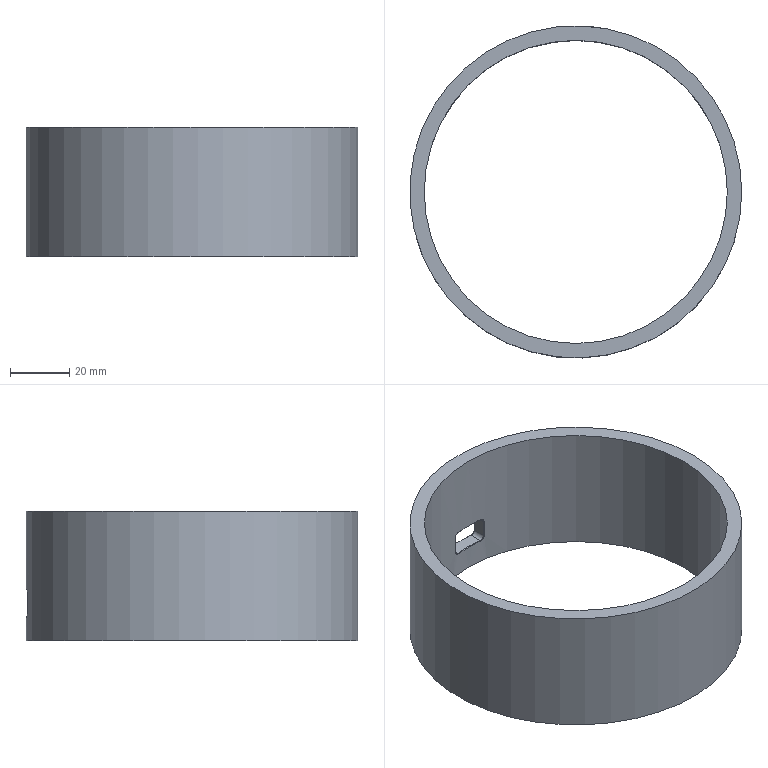NC program | NX | posted with a generic post | part box 112.5 x 112.5 x 44 mm
Whole program:
N10 G17 G21 G94 G90
(ZLEVEL_PROFILE_COPY , TOOL : D6)
N12 T04 M6
N14 G54
N16 G17 G0 G90 X1.72 Y10.5 B0. C0. S9500 M3
N18 G43 Z30. H4
N20 Z1.5
N22 G94 G1 X-3.75 Z1.213 F1500.
N24 Y8. Z1.082
N26 X3.75 Z0.689
N28 Y10.5 Z0.558
N30 X-3.75 Z0.165
N32 Y8. Z0.034
N34 X3.75 Z-0.359
N36 Y10.5 Z-0.49
N38 X-3.75
N40 Y8.
N42 X3.75
N44 Y10.5
N46 X-3.75 Z-0.735
N48 Y8. Z-0.817
N50 X1.25 Z-0.98
N52 X3.75
N54 Y10.5
N56 X-3.75 Z-1.225
N58 Y8. Z-1.306
N60 X1.25 Z-1.47
N62 X3.75
N64 Y10.5
N66 X-3.75 Z-1.715
N68 Y8. Z-1.796
N70 X1.25 Z-1.96
N72 X3.75
N74 Y10.5
N76 X-3.75 Z-2.205
N78 Y8. Z-2.286
N80 X1.25 Z-2.45
N82 X3.75
N84 Y10.5
N86 X-3.75 Z-2.695
N88 Y8. Z-2.776
N90 X1.25 Z-2.939
N92 X3.75
N94 Y10.5
N96 X-3.75 Z-3.184
N98 Y8. Z-3.266
N100 X1.25 Z-3.429
N102 X3.75
N104 Y10.5
N106 X-3.75 Z-3.674
N108 Y8. Z-3.756
N110 X1.25 Z-3.919
N112 X3.75
N114 Y10.5
N116 X-3.75 Z-4.164
N118 Y8. Z-4.246
N120 X1.25 Z-4.409
N122 X3.75
N124 Y10.5
N126 X-3.75 Z-4.654
N128 Y8. Z-4.736
N130 X1.25 Z-4.899
N132 X3.75
N134 Y10.5
N136 X-3.75 Z-5.144
N138 Y8. Z-5.226
N140 X1.25 Z-5.389
N142 X3.75
N144 Y10.5
N146 X-3.75 Z-5.634
N148 Y8. Z-5.716
N150 X1.25 Z-5.879
N152 X3.75
N154 Y10.5
N156 X-3.75 Z-6.124
N158 Y8. Z-6.206
N160 X1.25 Z-6.369
N162 X3.75
N164 Y10.5
N166 X-3.75
N168 Y8.
N170 X1.25
N172 Z-4.869
N174 G0 Z30.
N176 M5
(ADAPTIVE_MILLING , TOOL : D3)
N178 T05 M6
N180 G54
N182 G17 G0 G90 X3.003 Y7.25 B0. C0. S9500 M3
N184 G43 Z30. H5
N186 Z-3.
N188 G94 G1 Z-6. F1100.
N190 X3.197 Y6.702
N192 G3 X3.482 Y6.5 R0.305
N194 X4.28 Y6.992 R8.824
N196 X4.728 Y7.468 R2.682
N198 X5.201 Y8.025 R6.211
N200 X5.25 Y8.282 R0.441
N202 X4.998 Y8.603 R0.332
N204 X4.665 Y8.494 Z-5.939 R0.34
N206 G1 X4.503 Y8.33 Z-5.9
N208 X3.436 Y7.253
N210 X3.325 Y7.141 Z-5.926
N212 X3.217 Y7.026 Z-5.953
N214 G3 X3.161 Y6.756 Z-6. R0.335
N216 X3.482 Y6.5 R0.332
N218 X4.637 Y7.198 R2.342
N220 X5.198 Y7.85 R3.491
N222 G1 X5.238 Y7.919
N224 X5.25 Y7.998
N226 Y8.185
N228 G3 X4.694 Y8.426 R0.33
N230 G1 X3.256 Y7.07
N232 G3 X3.482 Y6.5 R0.33
N234 X4.253 Y6.758 R1.37
N236 X5.179 Y7.65 R3.378
N238 G1 X5.232 Y7.733
N240 X5.25 Y7.831
N242 Y8.
N244 G3 X4.705 Y8.25 R0.33
N246 G1 X3.342 Y7.08
N248 G3 X3.557 Y6.5 R0.33
N250 X4.37 Y6.739 R1.314
N252 X5.195 Y7.518 R2.602
N254 G1 X5.239 Y7.592
N256 X5.25 Y7.678
N258 Y7.847
N260 G3 X4.708 Y8.1 R0.33
N262 G1 X3.495 Y7.083
N264 G3 X3.707 Y6.5 R0.33
N266 X4.472 Y6.709 R1.272
N268 X5.216 Y7.408 R2.046
N270 X5.25 Y7.692 R0.614
N272 X4.71 Y7.946 R0.33
N274 G1 X3.666 Y7.085
N276 G3 X3.876 Y6.5 R0.33
N278 X4.654 Y6.73 R1.279
N280 X5.223 Y7.288 R1.579
N282 X5.25 Y7.536 R0.598
N284 X4.718 Y7.797 R0.33
N286 G1 X3.805 Y7.091
N288 G3 X4.007 Y6.5 R0.33
N290 X4.863 Y6.778 R1.276
N292 X5.234 Y7.191 R1.054
N294 X5.25 Y7.399 R0.714
N296 X4.723 Y7.664 R0.33
N298 G1 X3.96 Y7.094
N300 G3 X4.157 Y6.5 R0.33
N302 X5.086 Y6.871 R1.197
N304 X5.25 Y7.272 R0.457
N306 X4.727 Y7.54 R0.33
N308 G1 X4.114 Y7.098
N310 G3 X4.307 Y6.5 R0.33
N312 X5.22 Y6.95 R0.989
N314 X5.25 Y7.174 R0.509
N316 X4.723 Y7.439 R0.33
N318 G1 X4.26 Y7.095
N320 G3 X4.457 Y6.5 R0.33
N322 X5.216 Y6.859 R0.817
N324 X5.25 Y7.068 R0.434
N326 X4.728 Y7.336 R0.33
N328 G1 X4.396 Y7.098
N330 G3 X4.589 Y6.5 R0.33
N332 X5.218 Y6.794 R0.656
N334 G1 X5.248 Y6.852
N336 X5.259 Y6.917
N338 X5.25 Y6.982
N340 G3 X4.732 Y7.253 R0.33
N342 G1 X4.602 Y7.164
N344 X4.475 Y7.07
N346 G3 X4.701 Y6.5 R0.33
N348 X5.208 Y6.72 R0.54
N350 G1 X5.242 Y6.777
N352 X5.257 Y6.842
N354 X5.25 Y6.907
N356 G3 X4.747 Y7.188 R0.33
N358 G1 X4.663 Y7.137
N360 X4.581 Y7.081
N362 G3 X4.795 Y6.5 R0.33
N364 X5.205 Y6.673 R0.429
N366 G1 X5.239 Y6.727
N368 X5.255 Y6.789
N370 X5.25 Y6.853
N372 G3 X4.583 Y6.674 R-0.358
N374 X4.889 Y6.5 R0.359
N376 X5.25 Y6.828 R0.32
N378 X4.666 Y6.928 R0.301
N380 X5.009 Y6.508 R0.316
N382 G1 X5.027 Y6.514
N384 G3 X5.014 Y7.09 R0.303
N386 G1 X4.482 Y7.25
N388 Z-3.
N390 G0 Z30.
N392 X4.5 Y9.771
N394 Z-3.
N396 G1 Z-6.
N398 X5.04 Y9.944
N400 G3 X5.25 Y10.232 R0.305
N402 X4.758 Y11.03 R8.84
N404 X4.282 Y11.478 R2.677
N406 X3.725 Y11.951 R6.151
N408 X3.468 Y12. R0.441
N410 X3.147 Y11.748 R0.332
N412 X3.256 Y11.415 Z-5.939 R0.34
N414 G1 X3.42 Y11.253 Z-5.9
N416 X4.497 Y10.186
N418 X4.609 Y10.075 Z-5.926
N420 X4.724 Y9.967 Z-5.953
N422 G3 X4.994 Y9.911 Z-6. R0.335
N424 X5.25 Y10.232 R0.332
N426 X4.592 Y11.346 R2.271
N428 X3.916 Y11.938 R3.891
N430 G1 X3.84 Y11.986
N432 X3.752 Y12.
N434 X3.564
N436 G3 X3.324 Y11.444 R0.33
N438 G1 X4.68 Y10.006
N440 G3 X5.25 Y10.232 R0.33
N442 X5.002 Y10.987 R1.355
N444 X4.1 Y11.929 R3.388
N446 G1 X4.017 Y11.983
N448 X3.919 Y12.
N450 X3.75
N452 G3 X3.5 Y11.455 R0.33
N454 G1 X4.67 Y10.092
N456 G3 X5.25 Y10.307 R0.33
N458 X5.011 Y11.12 R1.315
N460 X4.232 Y11.945 R2.621
N462 G1 X4.158 Y11.989
N464 X4.072 Y12.
N466 X3.903
N468 G3 X3.65 Y11.458 R0.33
N470 G1 X4.667 Y10.245
N472 G3 X5.25 Y10.457 R0.33
N474 X5.04 Y11.222 R1.269
N476 X4.342 Y11.966 R2.047
N478 X4.058 Y12. R0.614
N480 X3.804 Y11.46 R0.33
N482 G1 X4.666 Y10.416
N484 G3 X5.25 Y10.626 R0.33
N486 X5.02 Y11.404 R1.279
N488 X4.462 Y11.973 R1.583
N490 X4.213 Y12. R0.597
N492 X3.954 Y11.465 R0.33
N494 G1 X4.661 Y10.572
N496 G3 X5.25 Y10.776 R0.33
N498 X4.983 Y11.597 R1.258
N500 X4.558 Y11.984 R1.07
N502 X4.351 Y12. R0.716
N504 X4.086 Y11.473 R0.33
N506 G1 X4.656 Y10.71
N508 G3 X5.25 Y10.907 R0.33
N510 X4.7 Y11.971 R1.184
N512 X4.477 Y12. R0.52
N514 X4.21 Y11.477 R0.33
N516 G1 X4.653 Y10.864
N518 G3 X5.25 Y11.057 R0.33
N520 X4.799 Y11.97 R0.99
N522 X4.576 Y12. R0.509
N524 X4.311 Y11.473 R0.33
N526 G1 X4.655 Y11.01
N528 G3 X5.25 Y11.207 R0.33
N530 X4.89 Y11.966 R0.82
N532 X4.682 Y12. R0.433
N534 X4.414 Y11.477 R0.33
N536 G1 X4.652 Y11.146
N538 G3 X5.25 Y11.339 R0.33
N540 X4.956 Y11.968 R0.657
N542 G1 X4.897 Y11.998
N544 X4.833 Y12.009
N546 X4.768 Y12.
N548 G3 X4.497 Y11.481 R0.33
N550 G1 X4.586 Y11.351
N552 X4.68 Y11.224
N554 G3 X5.25 Y11.451 R0.33
N556 X5.029 Y11.958 R0.541
N558 G1 X4.973 Y11.992
N560 X4.908 Y12.007
N562 X4.843 Y12.
N564 G3 X4.562 Y11.496 R0.33
N566 G1 X4.614 Y11.412
N568 X4.669 Y11.331
N570 G3 X5.25 Y11.545 R0.33
N572 X5.061 Y11.964 R0.421
N574 G1 X4.983 Y12.
N576 X4.897
N578 G3 X5.076 Y11.333 R-0.358
N580 X5.25 Y11.639 R0.359
N582 X4.922 Y12. R0.32
N584 X4.822 Y11.416 R0.301
N586 X5.242 Y11.759 R0.316
N588 G1 X5.236 Y11.777
N590 G3 X4.66 Y11.764 R0.303
N592 G1 X4.5 Y11.232
N594 Z-3.
N596 G0 Z30.
N598 X-3.003 Y11.25
N600 Z-3.
N602 G1 Z-6.
N604 X-3.197 Y11.798
N606 G3 X-3.482 Y12. R0.305
N608 X-4.28 Y11.508 R8.768
N610 X-4.728 Y11.031 R2.69
N612 X-5.201 Y10.475 R6.229
N614 X-5.25 Y10.218 R0.441
N616 X-4.998 Y9.897 R0.332
N618 X-4.665 Y10.006 Z-5.939 R0.34
N620 G1 X-4.503 Y10.17 Z-5.9
N622 X-3.436 Y11.247
N624 X-3.325 Y11.359 Z-5.926
N626 X-3.217 Y11.474 Z-5.953
N628 G3 X-3.161 Y11.744 Z-6. R0.335
N630 X-3.482 Y12. R0.332
N632 X-4.596 Y11.341 R2.266
N634 X-5.188 Y10.666 R3.896
N636 G1 X-5.236 Y10.59
N638 X-5.25 Y10.502
N640 Y10.314
N642 G3 X-4.694 Y10.074 R0.33
N644 G1 X-3.256 Y11.43
N646 G3 X-3.482 Y12. R0.33
N648 X-4.237 Y11.752 R1.354
N650 X-5.179 Y10.85 R3.409
N652 G1 X-5.233 Y10.767
N654 X-5.25 Y10.669
N656 Y10.5
N658 G3 X-4.705 Y10.25 R0.33
N660 G1 X-3.342 Y11.42
N662 G3 X-3.557 Y12. R0.33
N664 X-4.354 Y11.771 R1.297
N666 X-5.195 Y10.982 R2.635
N668 G1 X-5.239 Y10.908
N670 X-5.25 Y10.822
N672 Y10.653
N674 G3 X-4.708 Y10.4 R0.33
N676 G1 X-3.495 Y11.417
N678 G3 X-3.707 Y12. R0.33
N680 X-4.472 Y11.79 R1.271
N682 X-5.216 Y11.092 R2.049
N684 X-5.25 Y10.808 R0.614
N686 X-4.71 Y10.553 R0.33
N688 G1 X-3.666 Y11.416
N690 G3 X-3.876 Y12. R0.33
N692 X-4.654 Y11.77 R1.281
N694 X-5.223 Y11.212 R1.581
N696 X-5.25 Y10.963 R0.598
N698 X-4.718 Y10.702 R0.33
N700 G1 X-3.805 Y11.409
N702 G3 X-4.007 Y12. R0.33
N704 X-4.847 Y11.732 R1.266
N706 X-5.234 Y11.308 R1.07
N708 X-5.25 Y11.1 R0.715
N710 X-4.722 Y10.836 R0.33
N712 G1 X-3.96 Y11.406
N714 G3 X-4.157 Y12. R0.33
N716 X-5.221 Y11.45 R1.185
N718 X-5.25 Y11.227 R0.521
N720 X-4.727 Y10.96 R0.33
N722 G1 X-4.114 Y11.403
N724 G3 X-4.307 Y12. R0.33
N726 X-5.22 Y11.549 R0.99
N728 X-5.25 Y11.326 R0.509
N730 X-4.723 Y11.061 R0.33
N732 G1 X-4.26 Y11.405
N734 G3 X-4.457 Y12. R0.33
N736 X-5.216 Y11.641 R0.818
N738 X-5.25 Y11.432 R0.433
N740 X-4.727 Y11.164 R0.33
N742 G1 X-4.396 Y11.402
N744 G3 X-4.589 Y12. R0.33
N746 X-5.218 Y11.706 R0.657
N748 G1 X-5.248 Y11.648
N750 X-5.259 Y11.583
N752 X-5.25 Y11.518
N754 G3 X-4.732 Y11.247 R0.33
N756 G1 X-4.601 Y11.336
N758 X-4.475 Y11.43
N760 G3 X-4.701 Y12. R0.33
N762 X-5.208 Y11.78 R0.541
N764 X-5.25 Y11.574 R0.389
N766 X-4.699 Y11.329 R0.33
N768 G1 X-4.627 Y11.393
N770 X-4.558 Y11.461
N772 G3 X-4.814 Y12. R0.33
N774 X-5.241 Y11.741 R0.385
N776 G1 X-5.245 Y11.723
N778 X-5.248 Y11.704
N780 X-5.25 Y11.686
N782 Y11.648
N784 G3 X-4.56 Y11.779 R-0.358
N786 X-4.889 Y12. R0.357
N788 X-5.25 Y11.672 R0.32
N790 X-4.666 Y11.572 R0.301
N792 X-5.009 Y11.992 R0.316
N794 G1 X-5.027 Y11.986
N796 G3 X-5.014 Y11.41 R0.303
N798 G1 X-4.482 Y11.25
N800 Z-3.
N802 G0 Z30.
N804 X-4.5 Y8.729
N806 Z-3.
N808 G1 Z-6.
N810 X-5.04 Y8.556
N812 G3 X-5.25 Y8.268 R0.305
N814 X-4.747 Y7.455 R8.169
N816 X-4.31 Y7.046 R2.452
N818 X-3.741 Y6.559 R8.24
N820 X-3.468 Y6.5 R0.427
N822 X-3.147 Y6.752 R0.332
N824 X-3.256 Y7.085 Z-5.939 R0.34
N826 G1 X-3.42 Y7.247 Z-5.9
N828 X-4.497 Y8.314
N830 X-4.609 Y8.425 Z-5.926
N832 X-4.724 Y8.533 Z-5.953
N834 G3 X-4.994 Y8.589 Z-6. R0.335
N836 X-5.25 Y8.268 R0.332
N838 X-4.605 Y7.167 R2.24
N840 X-3.917 Y6.562 R3.951
N842 G1 X-3.84 Y6.514
N844 X-3.752 Y6.5
N846 X-3.564
N848 G3 X-3.324 Y7.056 R0.33
N850 G1 X-4.68 Y8.494
N852 G3 X-5.25 Y8.268 R0.33
N854 X-4.992 Y7.497 R1.367
N856 X-4.1 Y6.571 R3.398
N858 G1 X-4.017 Y6.517
N860 X-3.919 Y6.5
N862 X-3.751
N864 G3 X-3.5 Y7.045 R0.33
N866 G1 X-4.67 Y8.408
N868 G3 X-5.25 Y8.193 R0.33
N870 X-5.011 Y7.38 R1.312
N872 X-4.232 Y6.555 R2.621
N874 G1 X-4.158 Y6.511
N876 X-4.072 Y6.5
N878 X-3.903
N880 G3 X-3.65 Y7.042 R0.33
N882 G1 X-4.667 Y8.255
N884 G3 X-5.25 Y8.043 R0.33
N886 X-5.041 Y7.278 R1.274
N888 X-4.342 Y6.534 R2.051
N890 X-4.058 Y6.5 R0.615
N892 X-3.802 Y7.038 R0.33
N894 G1 X-4.664 Y8.1
N896 G3 X-5.25 Y7.893 R0.33
N898 X-5.02 Y7.096 R1.291
N900 X-4.462 Y6.527 R1.581
N902 X-4.213 Y6.5 R0.598
N904 X-3.952 Y7.032 R0.33
N906 G1 X-4.659 Y7.945
N908 G3 X-5.25 Y7.743 R0.33
N910 X-4.972 Y6.888 R1.278
N912 X-4.558 Y6.516 R1.059
N914 X-4.35 Y6.5 R0.713
N916 X-4.086 Y7.028 R0.33
N918 G1 X-4.656 Y7.79
N920 G3 X-5.25 Y7.593 R0.33
N922 X-4.905 Y6.691 R1.192
N924 X-4.59 Y6.5 R0.517
N926 G1 X-4.477
N928 G3 X-4.21 Y7.023 R0.33
N930 G1 X-4.653 Y7.636
N932 G3 X-5.25 Y7.443 R0.33
N934 X-4.799 Y6.53 R0.989
N936 X-4.576 Y6.5 R0.509
N938 X-4.311 Y7.027 R0.33
N940 G1 X-4.655 Y7.49
N942 G3 X-5.25 Y7.293 R0.33
N944 X-4.891 Y6.534 R0.818
N946 X-4.682 Y6.5 R0.433
N948 X-4.414 Y7.023 R0.33
N950 G1 X-4.652 Y7.354
N952 G3 X-5.25 Y7.161 R0.33
N954 X-4.956 Y6.532 R0.657
N956 G1 X-4.898 Y6.502
N958 X-4.833 Y6.491
N960 X-4.768 Y6.5
N962 G3 X-4.497 Y7.018 R0.33
N964 G1 X-4.586 Y7.149
N966 X-4.68 Y7.275
N968 G3 X-5.25 Y7.049 R0.33
N970 X-5.029 Y6.542 R0.54
N972 X-4.824 Y6.5 R0.39
N974 X-4.562 Y7.031 R0.33
N976 G1 X-4.625 Y7.114
N978 X-4.692 Y7.194
N980 G3 X-5.25 Y6.955 R0.33
N982 X-5.077 Y6.545 R0.429
N984 G1 X-5.024 Y6.511
N986 X-4.962 Y6.495
N988 X-4.898 Y6.5
N990 G3 X-5.029 Y7.19 R-0.358
N992 X-5.25 Y6.861 R0.357
N994 X-4.922 Y6.5 R0.32
N996 X-4.822 Y7.084 R0.301
N998 X-5.242 Y6.741 R0.316
N1000 G1 X-5.236 Y6.723
N1002 G3 X-4.66 Y6.736 R0.303
N1004 G1 X-4.5 Y7.268
N1006 Z-3.
N1008 G0 Z30.
(ZLEVEL_PROFILE , TOOL : D3)
N1010 X4.511 Y11.4
N1012 Z-6.369
N1014 G1 X5.1 Y11.74 F1200.
N1016 G3 X5.25 Y12. R0.3
N1018 G1 X-5.25
N1020 Y6.5
N1022 X5.25
N1024 Y12.
N1026 G3 X4.99 Y11.85 R0.3
N1028 G1 X4.65 Y11.261
N1030 G0 Z30.
N1032 M5
(PROFILE_3D , TOOL : D6A45)
N1034 T07 M6
N1036 G54
N1038 G17 G0 G90 X3.902 Y7.257 B0. C0. S9500 M3
N1040 G43 Z30. H7
N1042 Z-0.27
N1044 G94 G1 Z-1.77 F1250.
N1046 X4.641 Y6.288
N1048 G3 X5.195 Y6.057 R0.6
N1050 G1 X5.41 Y6.085 Z-1.785
N1052 X5.68 Y6.287 Z-1.914
N1054 X5.722 Y6.389 Z-1.955
N1056 X5.723 Y12.112 Z-1.942
N1058 X5.681 Y12.213
N1060 X5.613 Y12.3 Z-1.905
N1062 X5.52 Y12.37 Z-1.866
N1064 X5.41 Y12.415 Z-1.826
N1066 X5.194 Y12.443 Z-1.754
N1068 X1.766 Z-1.528
N1070 X-1.766
N1072 X-5.195 Z-1.77
N1074 X-5.41 Y12.415 Z-1.785
N1076 X-5.68 Y12.213 Z-1.914
N1078 X-5.722 Y12.111 Z-1.955
N1080 X-5.75 Y11.901 Z-1.968
N1082 Y6.598 Z-1.943
N1084 X-5.723 Y6.388 Z-1.942
N1086 X-5.681 Y6.287
N1088 X-5.613 Y6.2 Z-1.905
N1090 X-5.52 Y6.13 Z-1.866
N1092 X-5.41 Y6.085 Z-1.826
N1094 X-5.194 Y6.057 Z-1.754
N1096 X-1.766 Z-1.528
N1098 X1.766
N1100 X5.195 Z-1.77
N1102 G3 X5.715 Y6.357 R0.6
N1104 G1 X4.55 Y7.257
N1106 Z-0.27
N1108 G0 Z30.
N1110 M5
(FIXED_CONTOUR , TOOL : D4_LOLLIPOP)
N1112 T06 M6
N1114 G54
N1116 G17 G0 G90 X0. Y9.25 B0. C0. S9500 M3
N1118 G43 Z30. H6
N1120 Z-5.171
N1122 G94 G1 X-5.243 Y12. Z-8.486 F1250.
N1124 Y6.499
N1126 X-5.222 Y6.428 Z-8.476
N1128 X-5.171 Y6.386 Z-8.449
N1130 X-5.119 Z-8.412
N1132 X-5.086 Y6.414 Z-8.373
N1134 X-5.106 Z-8.375
N1136 X-3.832 Z-8.261
N1138 X-2.556 Z-8.179
N1140 X-1.279 Z-8.131
N1142 X0. Z-8.114
N1144 X1.279 Z-8.131
N1146 X2.556 Z-8.179
N1148 X3.832 Z-8.261
N1150 X5.099 Z-8.374
N1152 X5.096 Y6.397 Z-8.392
N1154 X5.116 Y6.386 Z-8.411
N1156 X5.171 Y6.387 Z-8.449
N1158 X5.222 Y6.428 Z-8.476
N1160 X5.243 Y6.5 Z-8.486
N1162 Y12.001
N1164 X5.222 Y12.072 Z-8.476
N1166 X5.171 Y12.114 Z-8.449
N1168 X5.119 Z-8.412
N1170 X5.086 Y12.086 Z-8.373
N1172 X5.106 Z-8.375
N1174 X3.832 Z-8.261
N1176 X2.556 Z-8.179
N1178 X1.279 Z-8.131
N1180 X0. Z-8.114
N1182 X-1.279 Z-8.131
N1184 X-2.556 Z-8.179
N1186 X-3.832 Z-8.261
N1188 X-5.099 Z-8.374
N1190 X-5.096 Y12.103 Z-8.392
N1192 X-5.116 Y12.114 Z-8.411
N1194 X-5.171 Y12.113 Z-8.449
N1196 X-5.222 Y12.072 Z-8.476
N1198 X-5.243 Y12. Z-8.486
N1200 X0. Y9.25 Z-5.171
N1202 G0 Z30.
N1204 M5
N1206 M2